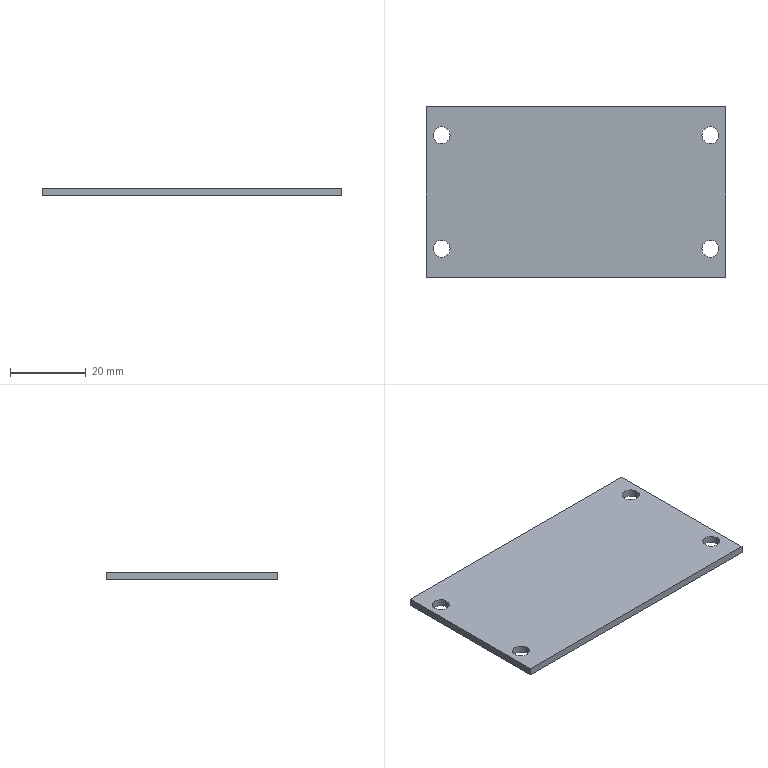Part | STEP file | Air switch plate 1 | 1 solid | 14 faces | box 79 x 45 x 2 mm | volume 6983 mm3 | cylinder 8 | plane 6 | commonest cylinder face diameters 4.5 x8
STEP:
#1=CARTESIAN_POINT('',(0.,0.,0.));
#2=DIRECTION('',(0.,0.,1.));
#3=DIRECTION('',(1.,0.,0.));
#4=AXIS2_PLACEMENT_3D('',#1,#2,#3);
#5=CARTESIAN_POINT('',(33.25,15.,2.));
#6=VERTEX_POINT('',#5);
#7=CARTESIAN_POINT('',(33.25,15.,0.));
#8=VERTEX_POINT('',#7);
#9=CARTESIAN_POINT('',(33.25,15.,2.));
#10=DIRECTION('',(0.,0.,-1.));
#11=VECTOR('',#10,1.);
#12=LINE('',#9,#11);
#13=CARTESIAN_POINT('',(35.5,15.,2.));
#14=DIRECTION('',(0.,0.,-1.));
#15=DIRECTION('',(-1.,0.,0.));
#16=AXIS2_PLACEMENT_3D('',#13,#14,#15);
#17=CYLINDRICAL_SURFACE('',#16,2.25);
#18=CARTESIAN_POINT('',(6.283,0.));
#19=DIRECTION('',(0.,1.));
#20=VECTOR('',#19,1.);
#21=LINE('',#18,#20);
#22=(GEOMETRIC_REPRESENTATION_CONTEXT(2)PARAMETRIC_REPRESENTATION_CONTEXT()REPRESENTATION_CONTEXT('',''));
#23=DEFINITIONAL_REPRESENTATION('',(#21),#22);
#24=PCURVE('',#17,#23);
#25=CARTESIAN_POINT('',(35.5,15.,2.));
#26=DIRECTION('',(0.,0.,-1.));
#27=DIRECTION('',(-1.,0.,0.));
#28=AXIS2_PLACEMENT_3D('',#25,#26,#27);
#29=CYLINDRICAL_SURFACE('',#28,2.25);
#30=CARTESIAN_POINT('',(0.,0.));
#31=DIRECTION('',(0.,1.));
#32=VECTOR('',#31,1.);
#33=LINE('',#30,#32);
#34=(GEOMETRIC_REPRESENTATION_CONTEXT(2)PARAMETRIC_REPRESENTATION_CONTEXT()REPRESENTATION_CONTEXT('',''));
#35=DEFINITIONAL_REPRESENTATION('',(#33),#34);
#36=PCURVE('',#29,#35);
#37=SURFACE_CURVE('',#12,(#24,#36),.PCURVE_S1.);
#38=EDGE_CURVE('',#6,#8,#37,.T.);
#39=ORIENTED_EDGE('',*,*,#38,.T.);
#40=CARTESIAN_POINT('',(37.75,15.,0.));
#41=VERTEX_POINT('',#40);
#42=CARTESIAN_POINT('',(35.5,15.,0.));
#43=DIRECTION('',(0.,0.,1.));
#44=DIRECTION('',(-1.,0.,0.));
#45=AXIS2_PLACEMENT_3D('',#42,#43,#44);
#46=CIRCLE('',#45,2.25);
#47=CARTESIAN_POINT('',(6.283,2.));
#48=DIRECTION('',(-1.,0.));
#49=VECTOR('',#48,1.);
#50=LINE('',#47,#49);
#51=(GEOMETRIC_REPRESENTATION_CONTEXT(2)PARAMETRIC_REPRESENTATION_CONTEXT()REPRESENTATION_CONTEXT('',''));
#52=DEFINITIONAL_REPRESENTATION('',(#50),#51);
#53=PCURVE('',#17,#52);
#54=CARTESIAN_POINT('',(39.5,-22.5,0.));
#55=DIRECTION('',(0.,0.,1.));
#56=DIRECTION('',(1.,0.,0.));
#57=AXIS2_PLACEMENT_3D('',#54,#55,#56);
#58=PLANE('',#57);
#59=CARTESIAN_POINT('',(-4.,37.5));
#60=DIRECTION('',(-1.,0.));
#61=AXIS2_PLACEMENT_2D('',#59,#60);
#62=CIRCLE('',#61,2.25);
#63=(GEOMETRIC_REPRESENTATION_CONTEXT(2)PARAMETRIC_REPRESENTATION_CONTEXT()REPRESENTATION_CONTEXT('',''));
#64=DEFINITIONAL_REPRESENTATION('',(#62),#63);
#65=PCURVE('',#58,#64);
#66=SURFACE_CURVE('',#46,(#53,#65),.PCURVE_S1.);
#67=EDGE_CURVE('',#8,#41,#66,.T.);
#68=ORIENTED_EDGE('',*,*,#67,.T.);
#69=CARTESIAN_POINT('',(37.75,15.,2.));
#70=VERTEX_POINT('',#69);
#71=CARTESIAN_POINT('',(37.75,15.,2.));
#72=DIRECTION('',(0.,0.,-1.));
#73=VECTOR('',#72,1.);
#74=LINE('',#71,#73);
#75=CARTESIAN_POINT('',(3.142,0.));
#76=DIRECTION('',(0.,1.));
#77=VECTOR('',#76,1.);
#78=LINE('',#75,#77);
#79=(GEOMETRIC_REPRESENTATION_CONTEXT(2)PARAMETRIC_REPRESENTATION_CONTEXT()REPRESENTATION_CONTEXT('',''));
#80=DEFINITIONAL_REPRESENTATION('',(#78),#79);
#81=PCURVE('',#17,#80);
#82=CARTESIAN_POINT('',(3.142,0.));
#83=DIRECTION('',(0.,1.));
#84=VECTOR('',#83,1.);
#85=LINE('',#82,#84);
#86=(GEOMETRIC_REPRESENTATION_CONTEXT(2)PARAMETRIC_REPRESENTATION_CONTEXT()REPRESENTATION_CONTEXT('',''));
#87=DEFINITIONAL_REPRESENTATION('',(#85),#86);
#88=PCURVE('',#29,#87);
#89=SURFACE_CURVE('',#74,(#81,#88),.PCURVE_S1.);
#90=EDGE_CURVE('',#70,#41,#89,.T.);
#91=ORIENTED_EDGE('',*,*,#90,.F.);
#92=CARTESIAN_POINT('',(35.5,15.,2.));
#93=DIRECTION('',(0.,0.,-1.));
#94=DIRECTION('',(-1.,0.,0.));
#95=AXIS2_PLACEMENT_3D('',#92,#93,#94);
#96=CIRCLE('',#95,2.25);
#97=CARTESIAN_POINT('',(0.,0.));
#98=DIRECTION('',(1.,0.));
#99=VECTOR('',#98,1.);
#100=LINE('',#97,#99);
#101=(GEOMETRIC_REPRESENTATION_CONTEXT(2)PARAMETRIC_REPRESENTATION_CONTEXT()REPRESENTATION_CONTEXT('',''));
#102=DEFINITIONAL_REPRESENTATION('',(#100),#101);
#103=PCURVE('',#17,#102);
#104=CARTESIAN_POINT('',(39.5,-22.5,2.));
#105=DIRECTION('',(0.,0.,1.));
#106=DIRECTION('',(1.,0.,0.));
#107=AXIS2_PLACEMENT_3D('',#104,#105,#106);
#108=PLANE('',#107);
#109=CARTESIAN_POINT('',(-6.25,37.5));
#110=CARTESIAN_POINT('',(-6.25,41.397));
#111=CARTESIAN_POINT('',(-2.875,39.449));
#112=CARTESIAN_POINT('',(0.5,37.5));
#113=CARTESIAN_POINT('',(-2.875,35.551));
#114=CARTESIAN_POINT('',(-6.25,33.603));
#115=CARTESIAN_POINT('',(-6.25,37.5));
#116=(BOUNDED_CURVE()B_SPLINE_CURVE(2,(#109,#110,#111,#112,#113,#114,#115),.UNSPECIFIED.,.T.,.F.)B_SPLINE_CURVE_WITH_KNOTS((1,2,2,2,2,1),(-2.094,0.,2.094,4.189,6.283,8.378),.UNSPECIFIED.)CURVE()GEOMETRIC_REPRESENTATION_ITEM()RATIONAL_B_SPLINE_CURVE((1.,0.5,1.,0.5,1.,0.5,1.))REPRESENTATION_ITEM(''));
#117=(GEOMETRIC_REPRESENTATION_CONTEXT(2)PARAMETRIC_REPRESENTATION_CONTEXT()REPRESENTATION_CONTEXT('',''));
#118=DEFINITIONAL_REPRESENTATION('',(#116),#117);
#119=PCURVE('',#108,#118);
#120=SURFACE_CURVE('',#96,(#103,#119),.PCURVE_S1.);
#121=EDGE_CURVE('',#70,#6,#120,.T.);
#122=ORIENTED_EDGE('',*,*,#121,.T.);
#123=EDGE_LOOP('',(#39,#68,#91,#122));
#124=FACE_BOUND('',#123,.F.);
#125=ADVANCED_FACE('',(#124),#17,.F.);
#126=CARTESIAN_POINT('',(-37.75,-15.,2.));
#127=VERTEX_POINT('',#126);
#128=CARTESIAN_POINT('',(-37.75,-15.,0.));
#129=VERTEX_POINT('',#128);
#130=CARTESIAN_POINT('',(-37.75,-15.,2.));
#131=DIRECTION('',(0.,0.,-1.));
#132=VECTOR('',#131,1.);
#133=LINE('',#130,#132);
#134=CARTESIAN_POINT('',(-35.5,-15.,2.));
#135=DIRECTION('',(0.,0.,-1.));
#136=DIRECTION('',(-1.,0.,0.));
#137=AXIS2_PLACEMENT_3D('',#134,#135,#136);
#138=CYLINDRICAL_SURFACE('',#137,2.25);
#139=CARTESIAN_POINT('',(6.283,0.));
#140=DIRECTION('',(0.,1.));
#141=VECTOR('',#140,1.);
#142=LINE('',#139,#141);
#143=(GEOMETRIC_REPRESENTATION_CONTEXT(2)PARAMETRIC_REPRESENTATION_CONTEXT()REPRESENTATION_CONTEXT('',''));
#144=DEFINITIONAL_REPRESENTATION('',(#142),#143);
#145=PCURVE('',#138,#144);
#146=CARTESIAN_POINT('',(-35.5,-15.,2.));
#147=DIRECTION('',(0.,0.,-1.));
#148=DIRECTION('',(-1.,0.,0.));
#149=AXIS2_PLACEMENT_3D('',#146,#147,#148);
#150=CYLINDRICAL_SURFACE('',#149,2.25);
#151=CARTESIAN_POINT('',(0.,0.));
#152=DIRECTION('',(0.,1.));
#153=VECTOR('',#152,1.);
#154=LINE('',#151,#153);
#155=(GEOMETRIC_REPRESENTATION_CONTEXT(2)PARAMETRIC_REPRESENTATION_CONTEXT()REPRESENTATION_CONTEXT('',''));
#156=DEFINITIONAL_REPRESENTATION('',(#154),#155);
#157=PCURVE('',#150,#156);
#158=SURFACE_CURVE('',#133,(#145,#157),.PCURVE_S1.);
#159=EDGE_CURVE('',#127,#129,#158,.T.);
#160=ORIENTED_EDGE('',*,*,#159,.T.);
#161=CARTESIAN_POINT('',(-33.25,-15.,0.));
#162=VERTEX_POINT('',#161);
#163=CARTESIAN_POINT('',(-35.5,-15.,0.));
#164=DIRECTION('',(0.,0.,1.));
#165=DIRECTION('',(-1.,0.,0.));
#166=AXIS2_PLACEMENT_3D('',#163,#164,#165);
#167=CIRCLE('',#166,2.25);
#168=CARTESIAN_POINT('',(6.283,2.));
#169=DIRECTION('',(-1.,0.));
#170=VECTOR('',#169,1.);
#171=LINE('',#168,#170);
#172=(GEOMETRIC_REPRESENTATION_CONTEXT(2)PARAMETRIC_REPRESENTATION_CONTEXT()REPRESENTATION_CONTEXT('',''));
#173=DEFINITIONAL_REPRESENTATION('',(#171),#172);
#174=PCURVE('',#138,#173);
#175=CARTESIAN_POINT('',(-75.,7.5));
#176=DIRECTION('',(-1.,0.));
#177=AXIS2_PLACEMENT_2D('',#175,#176);
#178=CIRCLE('',#177,2.25);
#179=(GEOMETRIC_REPRESENTATION_CONTEXT(2)PARAMETRIC_REPRESENTATION_CONTEXT()REPRESENTATION_CONTEXT('',''));
#180=DEFINITIONAL_REPRESENTATION('',(#178),#179);
#181=PCURVE('',#58,#180);
#182=SURFACE_CURVE('',#167,(#174,#181),.PCURVE_S1.);
#183=EDGE_CURVE('',#129,#162,#182,.T.);
#184=ORIENTED_EDGE('',*,*,#183,.T.);
#185=CARTESIAN_POINT('',(-33.25,-15.,2.));
#186=VERTEX_POINT('',#185);
#187=CARTESIAN_POINT('',(-33.25,-15.,2.));
#188=DIRECTION('',(0.,0.,-1.));
#189=VECTOR('',#188,1.);
#190=LINE('',#187,#189);
#191=CARTESIAN_POINT('',(3.142,0.));
#192=DIRECTION('',(0.,1.));
#193=VECTOR('',#192,1.);
#194=LINE('',#191,#193);
#195=(GEOMETRIC_REPRESENTATION_CONTEXT(2)PARAMETRIC_REPRESENTATION_CONTEXT()REPRESENTATION_CONTEXT('',''));
#196=DEFINITIONAL_REPRESENTATION('',(#194),#195);
#197=PCURVE('',#138,#196);
#198=CARTESIAN_POINT('',(3.142,0.));
#199=DIRECTION('',(0.,1.));
#200=VECTOR('',#199,1.);
#201=LINE('',#198,#200);
#202=(GEOMETRIC_REPRESENTATION_CONTEXT(2)PARAMETRIC_REPRESENTATION_CONTEXT()REPRESENTATION_CONTEXT('',''));
#203=DEFINITIONAL_REPRESENTATION('',(#201),#202);
#204=PCURVE('',#150,#203);
#205=SURFACE_CURVE('',#190,(#197,#204),.PCURVE_S1.);
#206=EDGE_CURVE('',#186,#162,#205,.T.);
#207=ORIENTED_EDGE('',*,*,#206,.F.);
#208=CARTESIAN_POINT('',(-35.5,-15.,2.));
#209=DIRECTION('',(0.,0.,-1.));
#210=DIRECTION('',(-1.,0.,0.));
#211=AXIS2_PLACEMENT_3D('',#208,#209,#210);
#212=CIRCLE('',#211,2.25);
#213=CARTESIAN_POINT('',(0.,0.));
#214=DIRECTION('',(1.,0.));
#215=VECTOR('',#214,1.);
#216=LINE('',#213,#215);
#217=(GEOMETRIC_REPRESENTATION_CONTEXT(2)PARAMETRIC_REPRESENTATION_CONTEXT()REPRESENTATION_CONTEXT('',''));
#218=DEFINITIONAL_REPRESENTATION('',(#216),#217);
#219=PCURVE('',#138,#218);
#220=CARTESIAN_POINT('',(-77.25,7.5));
#221=CARTESIAN_POINT('',(-77.25,11.397));
#222=CARTESIAN_POINT('',(-73.875,9.449));
#223=CARTESIAN_POINT('',(-70.5,7.5));
#224=CARTESIAN_POINT('',(-73.875,5.551));
#225=CARTESIAN_POINT('',(-77.25,3.603));
#226=CARTESIAN_POINT('',(-77.25,7.5));
#227=(BOUNDED_CURVE()B_SPLINE_CURVE(2,(#220,#221,#222,#223,#224,#225,#226),.UNSPECIFIED.,.T.,.F.)B_SPLINE_CURVE_WITH_KNOTS((1,2,2,2,2,1),(-2.094,0.,2.094,4.189,6.283,8.378),.UNSPECIFIED.)CURVE()GEOMETRIC_REPRESENTATION_ITEM()RATIONAL_B_SPLINE_CURVE((1.,0.5,1.,0.5,1.,0.5,1.))REPRESENTATION_ITEM(''));
#228=(GEOMETRIC_REPRESENTATION_CONTEXT(2)PARAMETRIC_REPRESENTATION_CONTEXT()REPRESENTATION_CONTEXT('',''));
#229=DEFINITIONAL_REPRESENTATION('',(#227),#228);
#230=PCURVE('',#108,#229);
#231=SURFACE_CURVE('',#212,(#219,#230),.PCURVE_S1.);
#232=EDGE_CURVE('',#186,#127,#231,.T.);
#233=ORIENTED_EDGE('',*,*,#232,.T.);
#234=EDGE_LOOP('',(#160,#184,#207,#233));
#235=FACE_BOUND('',#234,.F.);
#236=ADVANCED_FACE('',(#235),#138,.F.);
#237=CARTESIAN_POINT('',(-37.75,15.,2.));
#238=VERTEX_POINT('',#237);
#239=CARTESIAN_POINT('',(-37.75,15.,0.));
#240=VERTEX_POINT('',#239);
#241=CARTESIAN_POINT('',(-37.75,15.,2.));
#242=DIRECTION('',(0.,0.,-1.));
#243=VECTOR('',#242,1.);
#244=LINE('',#241,#243);
#245=CARTESIAN_POINT('',(-35.5,15.,2.));
#246=DIRECTION('',(0.,0.,-1.));
#247=DIRECTION('',(-1.,0.,0.));
#248=AXIS2_PLACEMENT_3D('',#245,#246,#247);
#249=CYLINDRICAL_SURFACE('',#248,2.25);
#250=CARTESIAN_POINT('',(6.283,0.));
#251=DIRECTION('',(0.,1.));
#252=VECTOR('',#251,1.);
#253=LINE('',#250,#252);
#254=(GEOMETRIC_REPRESENTATION_CONTEXT(2)PARAMETRIC_REPRESENTATION_CONTEXT()REPRESENTATION_CONTEXT('',''));
#255=DEFINITIONAL_REPRESENTATION('',(#253),#254);
#256=PCURVE('',#249,#255);
#257=CARTESIAN_POINT('',(-35.5,15.,2.));
#258=DIRECTION('',(0.,0.,-1.));
#259=DIRECTION('',(-1.,0.,0.));
#260=AXIS2_PLACEMENT_3D('',#257,#258,#259);
#261=CYLINDRICAL_SURFACE('',#260,2.25);
#262=CARTESIAN_POINT('',(0.,0.));
#263=DIRECTION('',(0.,1.));
#264=VECTOR('',#263,1.);
#265=LINE('',#262,#264);
#266=(GEOMETRIC_REPRESENTATION_CONTEXT(2)PARAMETRIC_REPRESENTATION_CONTEXT()REPRESENTATION_CONTEXT('',''));
#267=DEFINITIONAL_REPRESENTATION('',(#265),#266);
#268=PCURVE('',#261,#267);
#269=SURFACE_CURVE('',#244,(#256,#268),.PCURVE_S1.);
#270=EDGE_CURVE('',#238,#240,#269,.T.);
#271=ORIENTED_EDGE('',*,*,#270,.T.);
#272=CARTESIAN_POINT('',(-33.25,15.,0.));
#273=VERTEX_POINT('',#272);
#274=CARTESIAN_POINT('',(-35.5,15.,0.));
#275=DIRECTION('',(0.,0.,1.));
#276=DIRECTION('',(-1.,0.,0.));
#277=AXIS2_PLACEMENT_3D('',#274,#275,#276);
#278=CIRCLE('',#277,2.25);
#279=CARTESIAN_POINT('',(6.283,2.));
#280=DIRECTION('',(-1.,0.));
#281=VECTOR('',#280,1.);
#282=LINE('',#279,#281);
#283=(GEOMETRIC_REPRESENTATION_CONTEXT(2)PARAMETRIC_REPRESENTATION_CONTEXT()REPRESENTATION_CONTEXT('',''));
#284=DEFINITIONAL_REPRESENTATION('',(#282),#283);
#285=PCURVE('',#249,#284);
#286=CARTESIAN_POINT('',(-75.,37.5));
#287=DIRECTION('',(-1.,0.));
#288=AXIS2_PLACEMENT_2D('',#286,#287);
#289=CIRCLE('',#288,2.25);
#290=(GEOMETRIC_REPRESENTATION_CONTEXT(2)PARAMETRIC_REPRESENTATION_CONTEXT()REPRESENTATION_CONTEXT('',''));
#291=DEFINITIONAL_REPRESENTATION('',(#289),#290);
#292=PCURVE('',#58,#291);
#293=SURFACE_CURVE('',#278,(#285,#292),.PCURVE_S1.);
#294=EDGE_CURVE('',#240,#273,#293,.T.);
#295=ORIENTED_EDGE('',*,*,#294,.T.);
#296=CARTESIAN_POINT('',(-33.25,15.,2.));
#297=VERTEX_POINT('',#296);
#298=CARTESIAN_POINT('',(-33.25,15.,2.));
#299=DIRECTION('',(0.,0.,-1.));
#300=VECTOR('',#299,1.);
#301=LINE('',#298,#300);
#302=CARTESIAN_POINT('',(3.142,0.));
#303=DIRECTION('',(0.,1.));
#304=VECTOR('',#303,1.);
#305=LINE('',#302,#304);
#306=(GEOMETRIC_REPRESENTATION_CONTEXT(2)PARAMETRIC_REPRESENTATION_CONTEXT()REPRESENTATION_CONTEXT('',''));
#307=DEFINITIONAL_REPRESENTATION('',(#305),#306);
#308=PCURVE('',#249,#307);
#309=CARTESIAN_POINT('',(3.142,0.));
#310=DIRECTION('',(0.,1.));
#311=VECTOR('',#310,1.);
#312=LINE('',#309,#311);
#313=(GEOMETRIC_REPRESENTATION_CONTEXT(2)PARAMETRIC_REPRESENTATION_CONTEXT()REPRESENTATION_CONTEXT('',''));
#314=DEFINITIONAL_REPRESENTATION('',(#312),#313);
#315=PCURVE('',#261,#314);
#316=SURFACE_CURVE('',#301,(#308,#315),.PCURVE_S1.);
#317=EDGE_CURVE('',#297,#273,#316,.T.);
#318=ORIENTED_EDGE('',*,*,#317,.F.);
#319=CARTESIAN_POINT('',(-35.5,15.,2.));
#320=DIRECTION('',(0.,0.,-1.));
#321=DIRECTION('',(-1.,0.,0.));
#322=AXIS2_PLACEMENT_3D('',#319,#320,#321);
#323=CIRCLE('',#322,2.25);
#324=CARTESIAN_POINT('',(0.,0.));
#325=DIRECTION('',(1.,0.));
#326=VECTOR('',#325,1.);
#327=LINE('',#324,#326);
#328=(GEOMETRIC_REPRESENTATION_CONTEXT(2)PARAMETRIC_REPRESENTATION_CONTEXT()REPRESENTATION_CONTEXT('',''));
#329=DEFINITIONAL_REPRESENTATION('',(#327),#328);
#330=PCURVE('',#249,#329);
#331=CARTESIAN_POINT('',(-77.25,37.5));
#332=CARTESIAN_POINT('',(-77.25,41.397));
#333=CARTESIAN_POINT('',(-73.875,39.449));
#334=CARTESIAN_POINT('',(-70.5,37.5));
#335=CARTESIAN_POINT('',(-73.875,35.551));
#336=CARTESIAN_POINT('',(-77.25,33.603));
#337=CARTESIAN_POINT('',(-77.25,37.5));
#338=(BOUNDED_CURVE()B_SPLINE_CURVE(2,(#331,#332,#333,#334,#335,#336,#337),.UNSPECIFIED.,.T.,.F.)B_SPLINE_CURVE_WITH_KNOTS((1,2,2,2,2,1),(-2.094,0.,2.094,4.189,6.283,8.378),.UNSPECIFIED.)CURVE()GEOMETRIC_REPRESENTATION_ITEM()RATIONAL_B_SPLINE_CURVE((1.,0.5,1.,0.5,1.,0.5,1.))REPRESENTATION_ITEM(''));
#339=(GEOMETRIC_REPRESENTATION_CONTEXT(2)PARAMETRIC_REPRESENTATION_CONTEXT()REPRESENTATION_CONTEXT('',''));
#340=DEFINITIONAL_REPRESENTATION('',(#338),#339);
#341=PCURVE('',#108,#340);
#342=SURFACE_CURVE('',#323,(#330,#341),.PCURVE_S1.);
#343=EDGE_CURVE('',#297,#238,#342,.T.);
#344=ORIENTED_EDGE('',*,*,#343,.T.);
#345=EDGE_LOOP('',(#271,#295,#318,#344));
#346=FACE_BOUND('',#345,.F.);
#347=ADVANCED_FACE('',(#346),#249,.F.);
#348=CARTESIAN_POINT('',(33.25,-15.,2.));
#349=VERTEX_POINT('',#348);
#350=CARTESIAN_POINT('',(33.25,-15.,0.));
#351=VERTEX_POINT('',#350);
#352=CARTESIAN_POINT('',(33.25,-15.,2.));
#353=DIRECTION('',(0.,0.,-1.));
#354=VECTOR('',#353,1.);
#355=LINE('',#352,#354);
#356=CARTESIAN_POINT('',(35.5,-15.,2.));
#357=DIRECTION('',(0.,0.,-1.));
#358=DIRECTION('',(-1.,0.,0.));
#359=AXIS2_PLACEMENT_3D('',#356,#357,#358);
#360=CYLINDRICAL_SURFACE('',#359,2.25);
#361=CARTESIAN_POINT('',(6.283,0.));
#362=DIRECTION('',(0.,1.));
#363=VECTOR('',#362,1.);
#364=LINE('',#361,#363);
#365=(GEOMETRIC_REPRESENTATION_CONTEXT(2)PARAMETRIC_REPRESENTATION_CONTEXT()REPRESENTATION_CONTEXT('',''));
#366=DEFINITIONAL_REPRESENTATION('',(#364),#365);
#367=PCURVE('',#360,#366);
#368=CARTESIAN_POINT('',(35.5,-15.,2.));
#369=DIRECTION('',(0.,0.,-1.));
#370=DIRECTION('',(-1.,0.,0.));
#371=AXIS2_PLACEMENT_3D('',#368,#369,#370);
#372=CYLINDRICAL_SURFACE('',#371,2.25);
#373=CARTESIAN_POINT('',(0.,0.));
#374=DIRECTION('',(0.,1.));
#375=VECTOR('',#374,1.);
#376=LINE('',#373,#375);
#377=(GEOMETRIC_REPRESENTATION_CONTEXT(2)PARAMETRIC_REPRESENTATION_CONTEXT()REPRESENTATION_CONTEXT('',''));
#378=DEFINITIONAL_REPRESENTATION('',(#376),#377);
#379=PCURVE('',#372,#378);
#380=SURFACE_CURVE('',#355,(#367,#379),.PCURVE_S1.);
#381=EDGE_CURVE('',#349,#351,#380,.T.);
#382=ORIENTED_EDGE('',*,*,#381,.T.);
#383=CARTESIAN_POINT('',(37.75,-15.,0.));
#384=VERTEX_POINT('',#383);
#385=CARTESIAN_POINT('',(35.5,-15.,0.));
#386=DIRECTION('',(0.,0.,1.));
#387=DIRECTION('',(-1.,0.,0.));
#388=AXIS2_PLACEMENT_3D('',#385,#386,#387);
#389=CIRCLE('',#388,2.25);
#390=CARTESIAN_POINT('',(6.283,2.));
#391=DIRECTION('',(-1.,0.));
#392=VECTOR('',#391,1.);
#393=LINE('',#390,#392);
#394=(GEOMETRIC_REPRESENTATION_CONTEXT(2)PARAMETRIC_REPRESENTATION_CONTEXT()REPRESENTATION_CONTEXT('',''));
#395=DEFINITIONAL_REPRESENTATION('',(#393),#394);
#396=PCURVE('',#360,#395);
#397=CARTESIAN_POINT('',(-4.,7.5));
#398=DIRECTION('',(-1.,0.));
#399=AXIS2_PLACEMENT_2D('',#397,#398);
#400=CIRCLE('',#399,2.25);
#401=(GEOMETRIC_REPRESENTATION_CONTEXT(2)PARAMETRIC_REPRESENTATION_CONTEXT()REPRESENTATION_CONTEXT('',''));
#402=DEFINITIONAL_REPRESENTATION('',(#400),#401);
#403=PCURVE('',#58,#402);
#404=SURFACE_CURVE('',#389,(#396,#403),.PCURVE_S1.);
#405=EDGE_CURVE('',#351,#384,#404,.T.);
#406=ORIENTED_EDGE('',*,*,#405,.T.);
#407=CARTESIAN_POINT('',(37.75,-15.,2.));
#408=VERTEX_POINT('',#407);
#409=CARTESIAN_POINT('',(37.75,-15.,2.));
#410=DIRECTION('',(0.,0.,-1.));
#411=VECTOR('',#410,1.);
#412=LINE('',#409,#411);
#413=CARTESIAN_POINT('',(3.142,0.));
#414=DIRECTION('',(0.,1.));
#415=VECTOR('',#414,1.);
#416=LINE('',#413,#415);
#417=(GEOMETRIC_REPRESENTATION_CONTEXT(2)PARAMETRIC_REPRESENTATION_CONTEXT()REPRESENTATION_CONTEXT('',''));
#418=DEFINITIONAL_REPRESENTATION('',(#416),#417);
#419=PCURVE('',#360,#418);
#420=CARTESIAN_POINT('',(3.142,0.));
#421=DIRECTION('',(0.,1.));
#422=VECTOR('',#421,1.);
#423=LINE('',#420,#422);
#424=(GEOMETRIC_REPRESENTATION_CONTEXT(2)PARAMETRIC_REPRESENTATION_CONTEXT()REPRESENTATION_CONTEXT('',''));
#425=DEFINITIONAL_REPRESENTATION('',(#423),#424);
#426=PCURVE('',#372,#425);
#427=SURFACE_CURVE('',#412,(#419,#426),.PCURVE_S1.);
#428=EDGE_CURVE('',#408,#384,#427,.T.);
#429=ORIENTED_EDGE('',*,*,#428,.F.);
#430=CARTESIAN_POINT('',(35.5,-15.,2.));
#431=DIRECTION('',(0.,0.,-1.));
#432=DIRECTION('',(-1.,0.,0.));
#433=AXIS2_PLACEMENT_3D('',#430,#431,#432);
#434=CIRCLE('',#433,2.25);
#435=CARTESIAN_POINT('',(0.,0.));
#436=DIRECTION('',(1.,0.));
#437=VECTOR('',#436,1.);
#438=LINE('',#435,#437);
#439=(GEOMETRIC_REPRESENTATION_CONTEXT(2)PARAMETRIC_REPRESENTATION_CONTEXT()REPRESENTATION_CONTEXT('',''));
#440=DEFINITIONAL_REPRESENTATION('',(#438),#439);
#441=PCURVE('',#360,#440);
#442=CARTESIAN_POINT('',(-6.25,7.5));
#443=CARTESIAN_POINT('',(-6.25,11.397));
#444=CARTESIAN_POINT('',(-2.875,9.449));
#445=CARTESIAN_POINT('',(0.5,7.5));
#446=CARTESIAN_POINT('',(-2.875,5.551));
#447=CARTESIAN_POINT('',(-6.25,3.603));
#448=CARTESIAN_POINT('',(-6.25,7.5));
#449=(BOUNDED_CURVE()B_SPLINE_CURVE(2,(#442,#443,#444,#445,#446,#447,#448),.UNSPECIFIED.,.T.,.F.)B_SPLINE_CURVE_WITH_KNOTS((1,2,2,2,2,1),(-2.094,0.,2.094,4.189,6.283,8.378),.UNSPECIFIED.)CURVE()GEOMETRIC_REPRESENTATION_ITEM()RATIONAL_B_SPLINE_CURVE((1.,0.5,1.,0.5,1.,0.5,1.))REPRESENTATION_ITEM(''));
#450=(GEOMETRIC_REPRESENTATION_CONTEXT(2)PARAMETRIC_REPRESENTATION_CONTEXT()REPRESENTATION_CONTEXT('',''));
#451=DEFINITIONAL_REPRESENTATION('',(#449),#450);
#452=PCURVE('',#108,#451);
#453=SURFACE_CURVE('',#434,(#441,#452),.PCURVE_S1.);
#454=EDGE_CURVE('',#408,#349,#453,.T.);
#455=ORIENTED_EDGE('',*,*,#454,.T.);
#456=EDGE_LOOP('',(#382,#406,#429,#455));
#457=FACE_BOUND('',#456,.F.);
#458=ADVANCED_FACE('',(#457),#360,.F.);
#459=CARTESIAN_POINT('',(35.5,15.,2.));
#460=DIRECTION('',(0.,0.,-1.));
#461=DIRECTION('',(-1.,0.,0.));
#462=AXIS2_PLACEMENT_3D('',#459,#460,#461);
#463=CIRCLE('',#462,2.25);
#464=CARTESIAN_POINT('',(-6.25,37.5));
#465=CARTESIAN_POINT('',(-6.25,41.397));
#466=CARTESIAN_POINT('',(-2.875,39.449));
#467=CARTESIAN_POINT('',(0.5,37.5));
#468=CARTESIAN_POINT('',(-2.875,35.551));
#469=CARTESIAN_POINT('',(-6.25,33.603));
#470=CARTESIAN_POINT('',(-6.25,37.5));
#471=(BOUNDED_CURVE()B_SPLINE_CURVE(2,(#464,#465,#466,#467,#468,#469,#470),.UNSPECIFIED.,.T.,.F.)B_SPLINE_CURVE_WITH_KNOTS((1,2,2,2,2,1),(-2.094,0.,2.094,4.189,6.283,8.378),.UNSPECIFIED.)CURVE()GEOMETRIC_REPRESENTATION_ITEM()RATIONAL_B_SPLINE_CURVE((1.,0.5,1.,0.5,1.,0.5,1.))REPRESENTATION_ITEM(''));
#472=(GEOMETRIC_REPRESENTATION_CONTEXT(2)PARAMETRIC_REPRESENTATION_CONTEXT()REPRESENTATION_CONTEXT('',''));
#473=DEFINITIONAL_REPRESENTATION('',(#471),#472);
#474=PCURVE('',#108,#473);
#475=CARTESIAN_POINT('',(0.,0.));
#476=DIRECTION('',(1.,0.));
#477=VECTOR('',#476,1.);
#478=LINE('',#475,#477);
#479=(GEOMETRIC_REPRESENTATION_CONTEXT(2)PARAMETRIC_REPRESENTATION_CONTEXT()REPRESENTATION_CONTEXT('',''));
#480=DEFINITIONAL_REPRESENTATION('',(#478),#479);
#481=PCURVE('',#29,#480);
#482=SURFACE_CURVE('',#463,(#474,#481),.PCURVE_S1.);
#483=EDGE_CURVE('',#6,#70,#482,.T.);
#484=ORIENTED_EDGE('',*,*,#483,.T.);
#485=ORIENTED_EDGE('',*,*,#121,.T.);
#486=EDGE_LOOP('',(#484,#485));
#487=FACE_BOUND('',#486,.T.);
#488=CARTESIAN_POINT('',(-35.5,-15.,2.));
#489=DIRECTION('',(0.,0.,-1.));
#490=DIRECTION('',(-1.,0.,0.));
#491=AXIS2_PLACEMENT_3D('',#488,#489,#490);
#492=CIRCLE('',#491,2.25);
#493=CARTESIAN_POINT('',(-77.25,7.5));
#494=CARTESIAN_POINT('',(-77.25,11.397));
#495=CARTESIAN_POINT('',(-73.875,9.449));
#496=CARTESIAN_POINT('',(-70.5,7.5));
#497=CARTESIAN_POINT('',(-73.875,5.551));
#498=CARTESIAN_POINT('',(-77.25,3.603));
#499=CARTESIAN_POINT('',(-77.25,7.5));
#500=(BOUNDED_CURVE()B_SPLINE_CURVE(2,(#493,#494,#495,#496,#497,#498,#499),.UNSPECIFIED.,.T.,.F.)B_SPLINE_CURVE_WITH_KNOTS((1,2,2,2,2,1),(-2.094,0.,2.094,4.189,6.283,8.378),.UNSPECIFIED.)CURVE()GEOMETRIC_REPRESENTATION_ITEM()RATIONAL_B_SPLINE_CURVE((1.,0.5,1.,0.5,1.,0.5,1.))REPRESENTATION_ITEM(''));
#501=(GEOMETRIC_REPRESENTATION_CONTEXT(2)PARAMETRIC_REPRESENTATION_CONTEXT()REPRESENTATION_CONTEXT('',''));
#502=DEFINITIONAL_REPRESENTATION('',(#500),#501);
#503=PCURVE('',#108,#502);
#504=CARTESIAN_POINT('',(0.,0.));
#505=DIRECTION('',(1.,0.));
#506=VECTOR('',#505,1.);
#507=LINE('',#504,#506);
#508=(GEOMETRIC_REPRESENTATION_CONTEXT(2)PARAMETRIC_REPRESENTATION_CONTEXT()REPRESENTATION_CONTEXT('',''));
#509=DEFINITIONAL_REPRESENTATION('',(#507),#508);
#510=PCURVE('',#150,#509);
#511=SURFACE_CURVE('',#492,(#503,#510),.PCURVE_S1.);
#512=EDGE_CURVE('',#127,#186,#511,.T.);
#513=ORIENTED_EDGE('',*,*,#512,.T.);
#514=ORIENTED_EDGE('',*,*,#232,.T.);
#515=EDGE_LOOP('',(#513,#514));
#516=FACE_BOUND('',#515,.T.);
#517=CARTESIAN_POINT('',(-39.5,22.5,2.));
#518=VERTEX_POINT('',#517);
#519=CARTESIAN_POINT('',(-39.5,-22.5,2.));
#520=VERTEX_POINT('',#519);
#521=CARTESIAN_POINT('',(-39.5,-22.5,2.));
#522=DIRECTION('',(0.,-1.,0.));
#523=VECTOR('',#522,1.);
#524=LINE('',#521,#523);
#525=CARTESIAN_POINT('',(-79.,0.));
#526=DIRECTION('',(0.,-1.));
#527=VECTOR('',#526,1.);
#528=LINE('',#525,#527);
#529=(GEOMETRIC_REPRESENTATION_CONTEXT(2)PARAMETRIC_REPRESENTATION_CONTEXT()REPRESENTATION_CONTEXT('',''));
#530=DEFINITIONAL_REPRESENTATION('',(#528),#529);
#531=PCURVE('',#108,#530);
#532=CARTESIAN_POINT('',(-39.5,22.5,2.));
#533=DIRECTION('',(1.,0.,0.));
#534=DIRECTION('',(0.,1.,0.));
#535=AXIS2_PLACEMENT_3D('',#532,#533,#534);
#536=PLANE('',#535);
#537=CARTESIAN_POINT('',(-45.,0.));
#538=DIRECTION('',(-1.,0.));
#539=VECTOR('',#538,1.);
#540=LINE('',#537,#539);
#541=(GEOMETRIC_REPRESENTATION_CONTEXT(2)PARAMETRIC_REPRESENTATION_CONTEXT()REPRESENTATION_CONTEXT('',''));
#542=DEFINITIONAL_REPRESENTATION('',(#540),#541);
#543=PCURVE('',#536,#542);
#544=SURFACE_CURVE('',#524,(#531,#543),.PCURVE_S1.);
#545=EDGE_CURVE('',#518,#520,#544,.T.);
#546=ORIENTED_EDGE('',*,*,#545,.T.);
#547=CARTESIAN_POINT('',(39.5,-22.5,2.));
#548=VERTEX_POINT('',#547);
#549=CARTESIAN_POINT('',(39.5,-22.5,2.));
#550=DIRECTION('',(1.,0.,0.));
#551=VECTOR('',#550,1.);
#552=LINE('',#549,#551);
#553=CARTESIAN_POINT('',(0.,0.));
#554=DIRECTION('',(1.,0.));
#555=VECTOR('',#554,1.);
#556=LINE('',#553,#555);
#557=(GEOMETRIC_REPRESENTATION_CONTEXT(2)PARAMETRIC_REPRESENTATION_CONTEXT()REPRESENTATION_CONTEXT('',''));
#558=DEFINITIONAL_REPRESENTATION('',(#556),#557);
#559=PCURVE('',#108,#558);
#560=CARTESIAN_POINT('',(-39.5,-22.5,2.));
#561=DIRECTION('',(0.,1.,0.));
#562=DIRECTION('',(0.,0.,1.));
#563=AXIS2_PLACEMENT_3D('',#560,#561,#562);
#564=PLANE('',#563);
#565=CARTESIAN_POINT('',(0.,79.));
#566=DIRECTION('',(0.,1.));
#567=VECTOR('',#566,1.);
#568=LINE('',#565,#567);
#569=(GEOMETRIC_REPRESENTATION_CONTEXT(2)PARAMETRIC_REPRESENTATION_CONTEXT()REPRESENTATION_CONTEXT('',''));
#570=DEFINITIONAL_REPRESENTATION('',(#568),#569);
#571=PCURVE('',#564,#570);
#572=SURFACE_CURVE('',#552,(#559,#571),.PCURVE_S1.);
#573=EDGE_CURVE('',#520,#548,#572,.T.);
#574=ORIENTED_EDGE('',*,*,#573,.T.);
#575=CARTESIAN_POINT('',(39.5,22.5,2.));
#576=VERTEX_POINT('',#575);
#577=CARTESIAN_POINT('',(39.5,-22.5,2.));
#578=DIRECTION('',(0.,1.,0.));
#579=VECTOR('',#578,1.);
#580=LINE('',#577,#579);
#581=CARTESIAN_POINT('',(0.,0.));
#582=DIRECTION('',(0.,1.));
#583=VECTOR('',#582,1.);
#584=LINE('',#581,#583);
#585=(GEOMETRIC_REPRESENTATION_CONTEXT(2)PARAMETRIC_REPRESENTATION_CONTEXT()REPRESENTATION_CONTEXT('',''));
#586=DEFINITIONAL_REPRESENTATION('',(#584),#585);
#587=PCURVE('',#108,#586);
#588=CARTESIAN_POINT('',(39.5,22.5,2.));
#589=DIRECTION('',(-1.,0.,0.));
#590=DIRECTION('',(0.,-1.,0.));
#591=AXIS2_PLACEMENT_3D('',#588,#589,#590);
#592=PLANE('',#591);
#593=CARTESIAN_POINT('',(45.,0.));
#594=DIRECTION('',(-1.,0.));
#595=VECTOR('',#594,1.);
#596=LINE('',#593,#595);
#597=(GEOMETRIC_REPRESENTATION_CONTEXT(2)PARAMETRIC_REPRESENTATION_CONTEXT()REPRESENTATION_CONTEXT('',''));
#598=DEFINITIONAL_REPRESENTATION('',(#596),#597);
#599=PCURVE('',#592,#598);
#600=SURFACE_CURVE('',#580,(#587,#599),.PCURVE_S1.);
#601=EDGE_CURVE('',#548,#576,#600,.T.);
#602=ORIENTED_EDGE('',*,*,#601,.T.);
#603=CARTESIAN_POINT('',(39.5,22.5,2.));
#604=DIRECTION('',(-1.,0.,0.));
#605=VECTOR('',#604,1.);
#606=LINE('',#603,#605);
#607=CARTESIAN_POINT('',(0.,45.));
#608=DIRECTION('',(-1.,0.));
#609=VECTOR('',#608,1.);
#610=LINE('',#607,#609);
#611=(GEOMETRIC_REPRESENTATION_CONTEXT(2)PARAMETRIC_REPRESENTATION_CONTEXT()REPRESENTATION_CONTEXT('',''));
#612=DEFINITIONAL_REPRESENTATION('',(#610),#611);
#613=PCURVE('',#108,#612);
#614=CARTESIAN_POINT('',(-39.5,22.5,2.));
#615=DIRECTION('',(0.,-1.,0.));
#616=DIRECTION('',(0.,0.,-1.));
#617=AXIS2_PLACEMENT_3D('',#614,#615,#616);
#618=PLANE('',#617);
#619=CARTESIAN_POINT('',(0.,79.));
#620=DIRECTION('',(0.,-1.));
#621=VECTOR('',#620,1.);
#622=LINE('',#619,#621);
#623=(GEOMETRIC_REPRESENTATION_CONTEXT(2)PARAMETRIC_REPRESENTATION_CONTEXT()REPRESENTATION_CONTEXT('',''));
#624=DEFINITIONAL_REPRESENTATION('',(#622),#623);
#625=PCURVE('',#618,#624);
#626=SURFACE_CURVE('',#606,(#613,#625),.PCURVE_S1.);
#627=EDGE_CURVE('',#576,#518,#626,.T.);
#628=ORIENTED_EDGE('',*,*,#627,.T.);
#629=EDGE_LOOP('',(#546,#574,#602,#628));
#630=FACE_BOUND('',#629,.T.);
#631=CARTESIAN_POINT('',(-35.5,15.,2.));
#632=DIRECTION('',(0.,0.,-1.));
#633=DIRECTION('',(-1.,0.,0.));
#634=AXIS2_PLACEMENT_3D('',#631,#632,#633);
#635=CIRCLE('',#634,2.25);
#636=CARTESIAN_POINT('',(-77.25,37.5));
#637=CARTESIAN_POINT('',(-77.25,41.397));
#638=CARTESIAN_POINT('',(-73.875,39.449));
#639=CARTESIAN_POINT('',(-70.5,37.5));
#640=CARTESIAN_POINT('',(-73.875,35.551));
#641=CARTESIAN_POINT('',(-77.25,33.603));
#642=CARTESIAN_POINT('',(-77.25,37.5));
#643=(BOUNDED_CURVE()B_SPLINE_CURVE(2,(#636,#637,#638,#639,#640,#641,#642),.UNSPECIFIED.,.T.,.F.)B_SPLINE_CURVE_WITH_KNOTS((1,2,2,2,2,1),(-2.094,0.,2.094,4.189,6.283,8.378),.UNSPECIFIED.)CURVE()GEOMETRIC_REPRESENTATION_ITEM()RATIONAL_B_SPLINE_CURVE((1.,0.5,1.,0.5,1.,0.5,1.))REPRESENTATION_ITEM(''));
#644=(GEOMETRIC_REPRESENTATION_CONTEXT(2)PARAMETRIC_REPRESENTATION_CONTEXT()REPRESENTATION_CONTEXT('',''));
#645=DEFINITIONAL_REPRESENTATION('',(#643),#644);
#646=PCURVE('',#108,#645);
#647=CARTESIAN_POINT('',(0.,0.));
#648=DIRECTION('',(1.,0.));
#649=VECTOR('',#648,1.);
#650=LINE('',#647,#649);
#651=(GEOMETRIC_REPRESENTATION_CONTEXT(2)PARAMETRIC_REPRESENTATION_CONTEXT()REPRESENTATION_CONTEXT('',''));
#652=DEFINITIONAL_REPRESENTATION('',(#650),#651);
#653=PCURVE('',#261,#652);
#654=SURFACE_CURVE('',#635,(#646,#653),.PCURVE_S1.);
#655=EDGE_CURVE('',#238,#297,#654,.T.);
#656=ORIENTED_EDGE('',*,*,#655,.T.);
#657=ORIENTED_EDGE('',*,*,#343,.T.);
#658=EDGE_LOOP('',(#656,#657));
#659=FACE_BOUND('',#658,.T.);
#660=CARTESIAN_POINT('',(35.5,-15.,2.));
#661=DIRECTION('',(0.,0.,-1.));
#662=DIRECTION('',(-1.,0.,0.));
#663=AXIS2_PLACEMENT_3D('',#660,#661,#662);
#664=CIRCLE('',#663,2.25);
#665=CARTESIAN_POINT('',(-6.25,7.5));
#666=CARTESIAN_POINT('',(-6.25,11.397));
#667=CARTESIAN_POINT('',(-2.875,9.449));
#668=CARTESIAN_POINT('',(0.5,7.5));
#669=CARTESIAN_POINT('',(-2.875,5.551));
#670=CARTESIAN_POINT('',(-6.25,3.603));
#671=CARTESIAN_POINT('',(-6.25,7.5));
#672=(BOUNDED_CURVE()B_SPLINE_CURVE(2,(#665,#666,#667,#668,#669,#670,#671),.UNSPECIFIED.,.T.,.F.)B_SPLINE_CURVE_WITH_KNOTS((1,2,2,2,2,1),(-2.094,0.,2.094,4.189,6.283,8.378),.UNSPECIFIED.)CURVE()GEOMETRIC_REPRESENTATION_ITEM()RATIONAL_B_SPLINE_CURVE((1.,0.5,1.,0.5,1.,0.5,1.))REPRESENTATION_ITEM(''));
#673=(GEOMETRIC_REPRESENTATION_CONTEXT(2)PARAMETRIC_REPRESENTATION_CONTEXT()REPRESENTATION_CONTEXT('',''));
#674=DEFINITIONAL_REPRESENTATION('',(#672),#673);
#675=PCURVE('',#108,#674);
#676=CARTESIAN_POINT('',(0.,0.));
#677=DIRECTION('',(1.,0.));
#678=VECTOR('',#677,1.);
#679=LINE('',#676,#678);
#680=(GEOMETRIC_REPRESENTATION_CONTEXT(2)PARAMETRIC_REPRESENTATION_CONTEXT()REPRESENTATION_CONTEXT('',''));
#681=DEFINITIONAL_REPRESENTATION('',(#679),#680);
#682=PCURVE('',#372,#681);
#683=SURFACE_CURVE('',#664,(#675,#682),.PCURVE_S1.);
#684=EDGE_CURVE('',#349,#408,#683,.T.);
#685=ORIENTED_EDGE('',*,*,#684,.T.);
#686=ORIENTED_EDGE('',*,*,#454,.T.);
#687=EDGE_LOOP('',(#685,#686));
#688=FACE_BOUND('',#687,.T.);
#689=ADVANCED_FACE('',(#487,#516,#630,#659,#688),#108,.T.);
#690=CARTESIAN_POINT('',(35.5,15.,0.));
#691=DIRECTION('',(0.,0.,1.));
#692=DIRECTION('',(-1.,0.,0.));
#693=AXIS2_PLACEMENT_3D('',#690,#691,#692);
#694=CIRCLE('',#693,2.25);
#695=CARTESIAN_POINT('',(6.283,2.));
#696=DIRECTION('',(-1.,0.));
#697=VECTOR('',#696,1.);
#698=LINE('',#695,#697);
#699=(GEOMETRIC_REPRESENTATION_CONTEXT(2)PARAMETRIC_REPRESENTATION_CONTEXT()REPRESENTATION_CONTEXT('',''));
#700=DEFINITIONAL_REPRESENTATION('',(#698),#699);
#701=PCURVE('',#29,#700);
#702=CARTESIAN_POINT('',(-4.,37.5));
#703=DIRECTION('',(-1.,0.));
#704=AXIS2_PLACEMENT_2D('',#702,#703);
#705=CIRCLE('',#704,2.25);
#706=(GEOMETRIC_REPRESENTATION_CONTEXT(2)PARAMETRIC_REPRESENTATION_CONTEXT()REPRESENTATION_CONTEXT('',''));
#707=DEFINITIONAL_REPRESENTATION('',(#705),#706);
#708=PCURVE('',#58,#707);
#709=SURFACE_CURVE('',#694,(#701,#708),.PCURVE_S1.);
#710=EDGE_CURVE('',#41,#8,#709,.T.);
#711=ORIENTED_EDGE('',*,*,#710,.T.);
#712=ORIENTED_EDGE('',*,*,#38,.F.);
#713=ORIENTED_EDGE('',*,*,#483,.T.);
#714=ORIENTED_EDGE('',*,*,#90,.T.);
#715=EDGE_LOOP('',(#711,#712,#713,#714));
#716=FACE_BOUND('',#715,.F.);
#717=ADVANCED_FACE('',(#716),#29,.F.);
#718=CARTESIAN_POINT('',(-35.5,-15.,0.));
#719=DIRECTION('',(0.,0.,1.));
#720=DIRECTION('',(-1.,0.,0.));
#721=AXIS2_PLACEMENT_3D('',#718,#719,#720);
#722=CIRCLE('',#721,2.25);
#723=CARTESIAN_POINT('',(6.283,2.));
#724=DIRECTION('',(-1.,0.));
#725=VECTOR('',#724,1.);
#726=LINE('',#723,#725);
#727=(GEOMETRIC_REPRESENTATION_CONTEXT(2)PARAMETRIC_REPRESENTATION_CONTEXT()REPRESENTATION_CONTEXT('',''));
#728=DEFINITIONAL_REPRESENTATION('',(#726),#727);
#729=PCURVE('',#150,#728);
#730=CARTESIAN_POINT('',(-75.,7.5));
#731=DIRECTION('',(-1.,0.));
#732=AXIS2_PLACEMENT_2D('',#730,#731);
#733=CIRCLE('',#732,2.25);
#734=(GEOMETRIC_REPRESENTATION_CONTEXT(2)PARAMETRIC_REPRESENTATION_CONTEXT()REPRESENTATION_CONTEXT('',''));
#735=DEFINITIONAL_REPRESENTATION('',(#733),#734);
#736=PCURVE('',#58,#735);
#737=SURFACE_CURVE('',#722,(#729,#736),.PCURVE_S1.);
#738=EDGE_CURVE('',#162,#129,#737,.T.);
#739=ORIENTED_EDGE('',*,*,#738,.T.);
#740=ORIENTED_EDGE('',*,*,#159,.F.);
#741=ORIENTED_EDGE('',*,*,#512,.T.);
#742=ORIENTED_EDGE('',*,*,#206,.T.);
#743=EDGE_LOOP('',(#739,#740,#741,#742));
#744=FACE_BOUND('',#743,.F.);
#745=ADVANCED_FACE('',(#744),#150,.F.);
#746=CARTESIAN_POINT('',(39.5,-22.5,0.));
#747=VERTEX_POINT('',#746);
#748=CARTESIAN_POINT('',(39.5,-22.5,2.));
#749=DIRECTION('',(0.,0.,-1.));
#750=VECTOR('',#749,1.);
#751=LINE('',#748,#750);
#752=CARTESIAN_POINT('',(0.,79.));
#753=DIRECTION('',(-1.,0.));
#754=VECTOR('',#753,1.);
#755=LINE('',#752,#754);
#756=(GEOMETRIC_REPRESENTATION_CONTEXT(2)PARAMETRIC_REPRESENTATION_CONTEXT()REPRESENTATION_CONTEXT('',''));
#757=DEFINITIONAL_REPRESENTATION('',(#755),#756);
#758=PCURVE('',#564,#757);
#759=CARTESIAN_POINT('',(45.,0.));
#760=DIRECTION('',(0.,-1.));
#761=VECTOR('',#760,1.);
#762=LINE('',#759,#761);
#763=(GEOMETRIC_REPRESENTATION_CONTEXT(2)PARAMETRIC_REPRESENTATION_CONTEXT()REPRESENTATION_CONTEXT('',''));
#764=DEFINITIONAL_REPRESENTATION('',(#762),#763);
#765=PCURVE('',#592,#764);
#766=SURFACE_CURVE('',#751,(#758,#765),.PCURVE_S1.);
#767=EDGE_CURVE('',#548,#747,#766,.T.);
#768=ORIENTED_EDGE('',*,*,#767,.F.);
#769=ORIENTED_EDGE('',*,*,#573,.F.);
#770=CARTESIAN_POINT('',(-39.5,-22.5,0.));
#771=VERTEX_POINT('',#770);
#772=CARTESIAN_POINT('',(-39.5,-22.5,2.));
#773=DIRECTION('',(0.,0.,1.));
#774=VECTOR('',#773,1.);
#775=LINE('',#772,#774);
#776=CARTESIAN_POINT('',(0.,0.));
#777=DIRECTION('',(1.,0.));
#778=VECTOR('',#777,1.);
#779=LINE('',#776,#778);
#780=(GEOMETRIC_REPRESENTATION_CONTEXT(2)PARAMETRIC_REPRESENTATION_CONTEXT()REPRESENTATION_CONTEXT('',''));
#781=DEFINITIONAL_REPRESENTATION('',(#779),#780);
#782=PCURVE('',#564,#781);
#783=CARTESIAN_POINT('',(-45.,0.));
#784=DIRECTION('',(0.,1.));
#785=VECTOR('',#784,1.);
#786=LINE('',#783,#785);
#787=(GEOMETRIC_REPRESENTATION_CONTEXT(2)PARAMETRIC_REPRESENTATION_CONTEXT()REPRESENTATION_CONTEXT('',''));
#788=DEFINITIONAL_REPRESENTATION('',(#786),#787);
#789=PCURVE('',#536,#788);
#790=SURFACE_CURVE('',#775,(#782,#789),.PCURVE_S1.);
#791=EDGE_CURVE('',#771,#520,#790,.T.);
#792=ORIENTED_EDGE('',*,*,#791,.F.);
#793=CARTESIAN_POINT('',(-39.5,-22.5,0.));
#794=DIRECTION('',(-1.,0.,0.));
#795=VECTOR('',#794,1.);
#796=LINE('',#793,#795);
#797=CARTESIAN_POINT('',(-2.,0.));
#798=DIRECTION('',(0.,-1.));
#799=VECTOR('',#798,1.);
#800=LINE('',#797,#799);
#801=(GEOMETRIC_REPRESENTATION_CONTEXT(2)PARAMETRIC_REPRESENTATION_CONTEXT()REPRESENTATION_CONTEXT('',''));
#802=DEFINITIONAL_REPRESENTATION('',(#800),#801);
#803=PCURVE('',#564,#802);
#804=CARTESIAN_POINT('',(-79.,0.));
#805=DIRECTION('',(-1.,0.));
#806=VECTOR('',#805,1.);
#807=LINE('',#804,#806);
#808=(GEOMETRIC_REPRESENTATION_CONTEXT(2)PARAMETRIC_REPRESENTATION_CONTEXT()REPRESENTATION_CONTEXT('',''));
#809=DEFINITIONAL_REPRESENTATION('',(#807),#808);
#810=PCURVE('',#58,#809);
#811=SURFACE_CURVE('',#796,(#803,#810),.PCURVE_S1.);
#812=EDGE_CURVE('',#747,#771,#811,.T.);
#813=ORIENTED_EDGE('',*,*,#812,.F.);
#814=EDGE_LOOP('',(#768,#769,#792,#813));
#815=FACE_BOUND('',#814,.T.);
#816=ADVANCED_FACE('',(#815),#564,.F.);
#817=ORIENTED_EDGE('',*,*,#791,.T.);
#818=ORIENTED_EDGE('',*,*,#545,.F.);
#819=CARTESIAN_POINT('',(-39.5,22.5,0.));
#820=VERTEX_POINT('',#819);
#821=CARTESIAN_POINT('',(-39.5,22.5,2.));
#822=DIRECTION('',(0.,0.,1.));
#823=VECTOR('',#822,1.);
#824=LINE('',#821,#823);
#825=CARTESIAN_POINT('',(0.,0.));
#826=DIRECTION('',(0.,1.));
#827=VECTOR('',#826,1.);
#828=LINE('',#825,#827);
#829=(GEOMETRIC_REPRESENTATION_CONTEXT(2)PARAMETRIC_REPRESENTATION_CONTEXT()REPRESENTATION_CONTEXT('',''));
#830=DEFINITIONAL_REPRESENTATION('',(#828),#829);
#831=PCURVE('',#536,#830);
#832=CARTESIAN_POINT('',(0.,0.));
#833=DIRECTION('',(-1.,0.));
#834=VECTOR('',#833,1.);
#835=LINE('',#832,#834);
#836=(GEOMETRIC_REPRESENTATION_CONTEXT(2)PARAMETRIC_REPRESENTATION_CONTEXT()REPRESENTATION_CONTEXT('',''));
#837=DEFINITIONAL_REPRESENTATION('',(#835),#836);
#838=PCURVE('',#618,#837);
#839=SURFACE_CURVE('',#824,(#831,#838),.PCURVE_S1.);
#840=EDGE_CURVE('',#820,#518,#839,.T.);
#841=ORIENTED_EDGE('',*,*,#840,.F.);
#842=CARTESIAN_POINT('',(-39.5,22.5,0.));
#843=DIRECTION('',(0.,1.,0.));
#844=VECTOR('',#843,1.);
#845=LINE('',#842,#844);
#846=CARTESIAN_POINT('',(0.,-2.));
#847=DIRECTION('',(1.,0.));
#848=VECTOR('',#847,1.);
#849=LINE('',#846,#848);
#850=(GEOMETRIC_REPRESENTATION_CONTEXT(2)PARAMETRIC_REPRESENTATION_CONTEXT()REPRESENTATION_CONTEXT('',''));
#851=DEFINITIONAL_REPRESENTATION('',(#849),#850);
#852=PCURVE('',#536,#851);
#853=CARTESIAN_POINT('',(-79.,45.));
#854=DIRECTION('',(0.,1.));
#855=VECTOR('',#854,1.);
#856=LINE('',#853,#855);
#857=(GEOMETRIC_REPRESENTATION_CONTEXT(2)PARAMETRIC_REPRESENTATION_CONTEXT()REPRESENTATION_CONTEXT('',''));
#858=DEFINITIONAL_REPRESENTATION('',(#856),#857);
#859=PCURVE('',#58,#858);
#860=SURFACE_CURVE('',#845,(#852,#859),.PCURVE_S1.);
#861=EDGE_CURVE('',#771,#820,#860,.T.);
#862=ORIENTED_EDGE('',*,*,#861,.F.);
#863=EDGE_LOOP('',(#817,#818,#841,#862));
#864=FACE_BOUND('',#863,.T.);
#865=ADVANCED_FACE('',(#864),#536,.F.);
#866=ORIENTED_EDGE('',*,*,#840,.T.);
#867=ORIENTED_EDGE('',*,*,#627,.F.);
#868=CARTESIAN_POINT('',(39.5,22.5,0.));
#869=VERTEX_POINT('',#868);
#870=CARTESIAN_POINT('',(39.5,22.5,2.));
#871=DIRECTION('',(0.,0.,1.));
#872=VECTOR('',#871,1.);
#873=LINE('',#870,#872);
#874=CARTESIAN_POINT('',(0.,79.));
#875=DIRECTION('',(-1.,0.));
#876=VECTOR('',#875,1.);
#877=LINE('',#874,#876);
#878=(GEOMETRIC_REPRESENTATION_CONTEXT(2)PARAMETRIC_REPRESENTATION_CONTEXT()REPRESENTATION_CONTEXT('',''));
#879=DEFINITIONAL_REPRESENTATION('',(#877),#878);
#880=PCURVE('',#618,#879);
#881=CARTESIAN_POINT('',(0.,0.));
#882=DIRECTION('',(0.,1.));
#883=VECTOR('',#882,1.);
#884=LINE('',#881,#883);
#885=(GEOMETRIC_REPRESENTATION_CONTEXT(2)PARAMETRIC_REPRESENTATION_CONTEXT()REPRESENTATION_CONTEXT('',''));
#886=DEFINITIONAL_REPRESENTATION('',(#884),#885);
#887=PCURVE('',#592,#886);
#888=SURFACE_CURVE('',#873,(#880,#887),.PCURVE_S1.);
#889=EDGE_CURVE('',#869,#576,#888,.T.);
#890=ORIENTED_EDGE('',*,*,#889,.F.);
#891=CARTESIAN_POINT('',(-39.5,22.5,0.));
#892=DIRECTION('',(1.,0.,0.));
#893=VECTOR('',#892,1.);
#894=LINE('',#891,#893);
#895=CARTESIAN_POINT('',(2.,0.));
#896=DIRECTION('',(0.,1.));
#897=VECTOR('',#896,1.);
#898=LINE('',#895,#897);
#899=(GEOMETRIC_REPRESENTATION_CONTEXT(2)PARAMETRIC_REPRESENTATION_CONTEXT()REPRESENTATION_CONTEXT('',''));
#900=DEFINITIONAL_REPRESENTATION('',(#898),#899);
#901=PCURVE('',#618,#900);
#902=CARTESIAN_POINT('',(-79.,45.));
#903=DIRECTION('',(1.,0.));
#904=VECTOR('',#903,1.);
#905=LINE('',#902,#904);
#906=(GEOMETRIC_REPRESENTATION_CONTEXT(2)PARAMETRIC_REPRESENTATION_CONTEXT()REPRESENTATION_CONTEXT('',''));
#907=DEFINITIONAL_REPRESENTATION('',(#905),#906);
#908=PCURVE('',#58,#907);
#909=SURFACE_CURVE('',#894,(#901,#908),.PCURVE_S1.);
#910=EDGE_CURVE('',#820,#869,#909,.T.);
#911=ORIENTED_EDGE('',*,*,#910,.F.);
#912=EDGE_LOOP('',(#866,#867,#890,#911));
#913=FACE_BOUND('',#912,.T.);
#914=ADVANCED_FACE('',(#913),#618,.F.);
#915=ORIENTED_EDGE('',*,*,#889,.T.);
#916=ORIENTED_EDGE('',*,*,#601,.F.);
#917=ORIENTED_EDGE('',*,*,#767,.T.);
#918=CARTESIAN_POINT('',(39.5,22.5,0.));
#919=DIRECTION('',(0.,-1.,0.));
#920=VECTOR('',#919,1.);
#921=LINE('',#918,#920);
#922=CARTESIAN_POINT('',(0.,-2.));
#923=DIRECTION('',(1.,0.));
#924=VECTOR('',#923,1.);
#925=LINE('',#922,#924);
#926=(GEOMETRIC_REPRESENTATION_CONTEXT(2)PARAMETRIC_REPRESENTATION_CONTEXT()REPRESENTATION_CONTEXT('',''));
#927=DEFINITIONAL_REPRESENTATION('',(#925),#926);
#928=PCURVE('',#592,#927);
#929=CARTESIAN_POINT('',(0.,45.));
#930=DIRECTION('',(0.,-1.));
#931=VECTOR('',#930,1.);
#932=LINE('',#929,#931);
#933=(GEOMETRIC_REPRESENTATION_CONTEXT(2)PARAMETRIC_REPRESENTATION_CONTEXT()REPRESENTATION_CONTEXT('',''));
#934=DEFINITIONAL_REPRESENTATION('',(#932),#933);
#935=PCURVE('',#58,#934);
#936=SURFACE_CURVE('',#921,(#928,#935),.PCURVE_S1.);
#937=EDGE_CURVE('',#869,#747,#936,.T.);
#938=ORIENTED_EDGE('',*,*,#937,.F.);
#939=EDGE_LOOP('',(#915,#916,#917,#938));
#940=FACE_BOUND('',#939,.T.);
#941=ADVANCED_FACE('',(#940),#592,.F.);
#942=CARTESIAN_POINT('',(-35.5,15.,0.));
#943=DIRECTION('',(0.,0.,1.));
#944=DIRECTION('',(-1.,0.,0.));
#945=AXIS2_PLACEMENT_3D('',#942,#943,#944);
#946=CIRCLE('',#945,2.25);
#947=CARTESIAN_POINT('',(6.283,2.));
#948=DIRECTION('',(-1.,0.));
#949=VECTOR('',#948,1.);
#950=LINE('',#947,#949);
#951=(GEOMETRIC_REPRESENTATION_CONTEXT(2)PARAMETRIC_REPRESENTATION_CONTEXT()REPRESENTATION_CONTEXT('',''));
#952=DEFINITIONAL_REPRESENTATION('',(#950),#951);
#953=PCURVE('',#261,#952);
#954=CARTESIAN_POINT('',(-75.,37.5));
#955=DIRECTION('',(-1.,0.));
#956=AXIS2_PLACEMENT_2D('',#954,#955);
#957=CIRCLE('',#956,2.25);
#958=(GEOMETRIC_REPRESENTATION_CONTEXT(2)PARAMETRIC_REPRESENTATION_CONTEXT()REPRESENTATION_CONTEXT('',''));
#959=DEFINITIONAL_REPRESENTATION('',(#957),#958);
#960=PCURVE('',#58,#959);
#961=SURFACE_CURVE('',#946,(#953,#960),.PCURVE_S1.);
#962=EDGE_CURVE('',#273,#240,#961,.T.);
#963=ORIENTED_EDGE('',*,*,#962,.T.);
#964=ORIENTED_EDGE('',*,*,#270,.F.);
#965=ORIENTED_EDGE('',*,*,#655,.T.);
#966=ORIENTED_EDGE('',*,*,#317,.T.);
#967=EDGE_LOOP('',(#963,#964,#965,#966));
#968=FACE_BOUND('',#967,.F.);
#969=ADVANCED_FACE('',(#968),#261,.F.);
#970=CARTESIAN_POINT('',(35.5,-15.,0.));
#971=DIRECTION('',(0.,0.,1.));
#972=DIRECTION('',(-1.,0.,0.));
#973=AXIS2_PLACEMENT_3D('',#970,#971,#972);
#974=CIRCLE('',#973,2.25);
#975=CARTESIAN_POINT('',(6.283,2.));
#976=DIRECTION('',(-1.,0.));
#977=VECTOR('',#976,1.);
#978=LINE('',#975,#977);
#979=(GEOMETRIC_REPRESENTATION_CONTEXT(2)PARAMETRIC_REPRESENTATION_CONTEXT()REPRESENTATION_CONTEXT('',''));
#980=DEFINITIONAL_REPRESENTATION('',(#978),#979);
#981=PCURVE('',#372,#980);
#982=CARTESIAN_POINT('',(-4.,7.5));
#983=DIRECTION('',(-1.,0.));
#984=AXIS2_PLACEMENT_2D('',#982,#983);
#985=CIRCLE('',#984,2.25);
#986=(GEOMETRIC_REPRESENTATION_CONTEXT(2)PARAMETRIC_REPRESENTATION_CONTEXT()REPRESENTATION_CONTEXT('',''));
#987=DEFINITIONAL_REPRESENTATION('',(#985),#986);
#988=PCURVE('',#58,#987);
#989=SURFACE_CURVE('',#974,(#981,#988),.PCURVE_S1.);
#990=EDGE_CURVE('',#384,#351,#989,.T.);
#991=ORIENTED_EDGE('',*,*,#990,.T.);
#992=ORIENTED_EDGE('',*,*,#381,.F.);
#993=ORIENTED_EDGE('',*,*,#684,.T.);
#994=ORIENTED_EDGE('',*,*,#428,.T.);
#995=EDGE_LOOP('',(#991,#992,#993,#994));
#996=FACE_BOUND('',#995,.F.);
#997=ADVANCED_FACE('',(#996),#372,.F.);
#998=ORIENTED_EDGE('',*,*,#67,.T.);
#999=ORIENTED_EDGE('',*,*,#710,.T.);
#1000=EDGE_LOOP('',(#998,#999));
#1001=FACE_BOUND('',#1000,.T.);
#1002=ORIENTED_EDGE('',*,*,#183,.T.);
#1003=ORIENTED_EDGE('',*,*,#738,.T.);
#1004=EDGE_LOOP('',(#1002,#1003));
#1005=FACE_BOUND('',#1004,.T.);
#1006=ORIENTED_EDGE('',*,*,#812,.T.);
#1007=ORIENTED_EDGE('',*,*,#861,.T.);
#1008=ORIENTED_EDGE('',*,*,#910,.T.);
#1009=ORIENTED_EDGE('',*,*,#937,.T.);
#1010=EDGE_LOOP('',(#1006,#1007,#1008,#1009));
#1011=FACE_BOUND('',#1010,.T.);
#1012=ORIENTED_EDGE('',*,*,#294,.T.);
#1013=ORIENTED_EDGE('',*,*,#962,.T.);
#1014=EDGE_LOOP('',(#1012,#1013));
#1015=FACE_BOUND('',#1014,.T.);
#1016=ORIENTED_EDGE('',*,*,#405,.T.);
#1017=ORIENTED_EDGE('',*,*,#990,.T.);
#1018=EDGE_LOOP('',(#1016,#1017));
#1019=FACE_BOUND('',#1018,.T.);
#1020=ADVANCED_FACE('',(#1001,#1005,#1011,#1015,#1019),#58,.F.);
#1021=CLOSED_SHELL('',(#125,#236,#347,#458,#689,#717,#745,#816,#865,#914,#941,#969,#997,#1020));
#1022=MANIFOLD_SOLID_BREP('',#1021);
#1023=(LENGTH_UNIT()NAMED_UNIT(*)SI_UNIT(.MILLI.,.METRE.));
#1024=UNCERTAINTY_MEASURE_WITH_UNIT(LENGTH_MEASURE(0.0000001),#1023,'','');
#1025=(NAMED_UNIT(*)PLANE_ANGLE_UNIT()SI_UNIT($,.RADIAN.));
#1026=(NAMED_UNIT(*)SI_UNIT($,.STERADIAN.)SOLID_ANGLE_UNIT());
#1027=(GEOMETRIC_REPRESENTATION_CONTEXT(3)GLOBAL_UNCERTAINTY_ASSIGNED_CONTEXT((#1024))GLOBAL_UNIT_ASSIGNED_CONTEXT((#1023,#1025,#1026))REPRESENTATION_CONTEXT('',''));
#1028=ADVANCED_BREP_SHAPE_REPRESENTATION('',(#4,#1022),#1027);